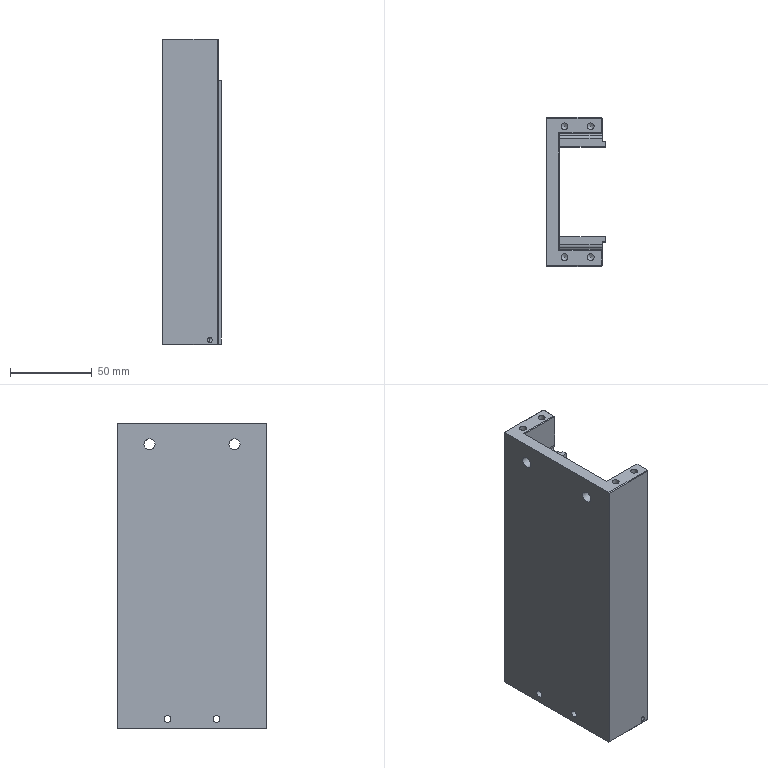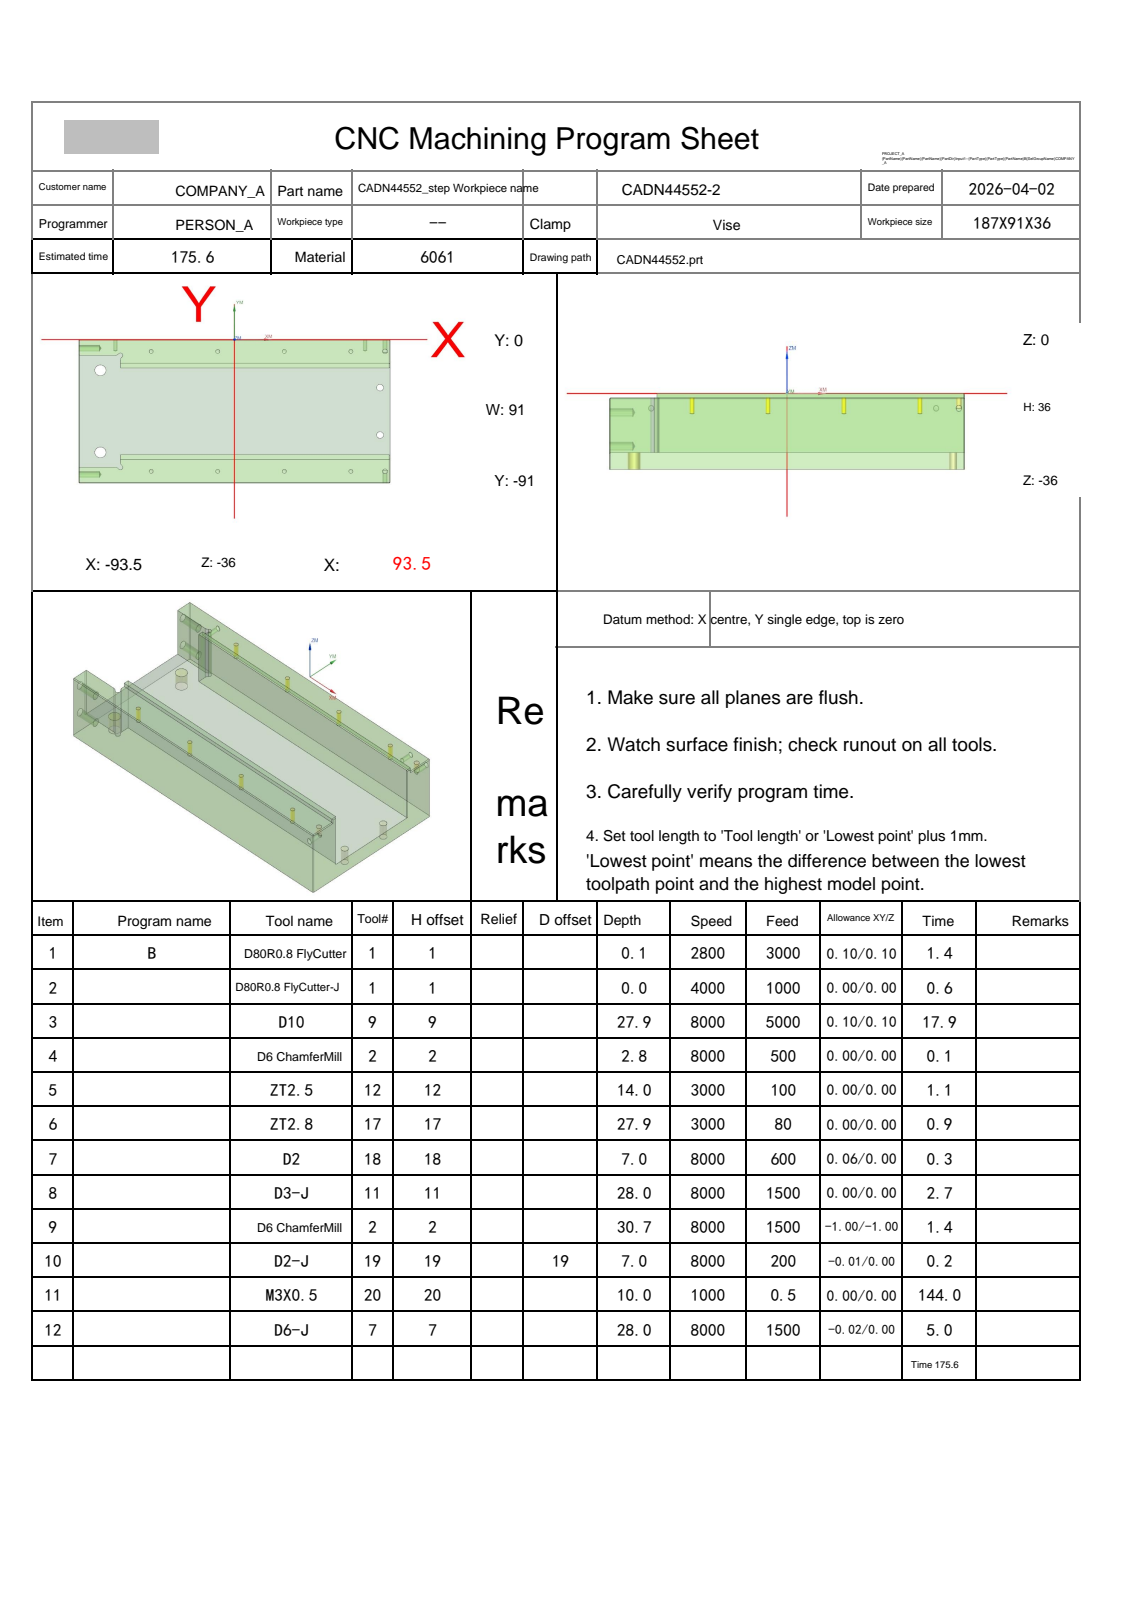NC program | NX | posted by the shop | part box 36 x 91 x 187 mm
Lines 5693 to 6699 of 12140:
N8 T11 M06
(D3-J  D=2.95 R=0. H=11 ce=0.00 di=0.00)
G00 G90 G54 X-74.719 Y-79.229 M03 S8000
G43 H11 Z20.
M08
Z-1.955
G01 X-74.718 Y-79.233 Z-2. F1500.
X-74.716 Y-79.243 Z-2.04
X-74.711 Y-79.26 Z-2.076
X-74.704 Y-79.281 Z-2.108
X-74.695 Y-79.306 Z-2.136
X-74.683 Y-79.333 Z-2.161
X-74.669 Y-79.362 Z-2.182
X-74.651 Y-79.392 Z-2.199
X-74.63 Y-79.421 Z-2.214
X-74.605 Y-79.448 Z-2.226
X-74.577 Y-79.473 Z-2.235
X-74.545 Y-79.494 Z-2.242
X-74.509 Y-79.511 Z-2.247
X-74.469 Y-79.521 Z-2.249
X-74.424 Y-79.525 Z-2.25
X-71.622
G02 X-68.52 Y-81.016 I0.0 J-3.975
G01 X-68.492 Y-81.034
X-68.466 Y-81.008
X-68.484 Y-80.98
G02 X-69.975 Y-77.877 I2.484 J3.103
G01 Y-75.076
X-69.989 Y-75.052 Z-2.251
X-70.03 Z-2.252
X-70.096 Y-75.076 Z-2.255
X-70.184 Y-75.12 Z-2.259
X-70.292 Y-75.183 Z-2.264
X-70.623 Y-75.411 Z-2.28
X-70.927 Y-75.64 Z-2.294
X-71.309 Y-75.946 Z-2.313
X-71.944 Y-76.503 Z-2.346
X-72.481 Y-77.019 Z-2.375
X-72.996 Y-77.555 Z-2.404
X-73.553 Y-78.19 Z-2.437
X-73.86 Y-78.572 Z-2.456
X-74.089 Y-78.876 Z-2.47
X-74.317 Y-79.208 Z-2.486
X-74.38 Y-79.316 Z-2.491
X-74.424 Y-79.404 Z-2.495
X-74.448 Y-79.47 Z-2.498
Y-79.511 Z-2.499
X-74.424 Y-79.525 Z-2.5
X-71.622
G02 X-68.52 Y-81.016 I0.0 J-3.975
G01 X-68.492 Y-81.034
X-68.466 Y-81.008
X-68.484 Y-80.98
G02 X-69.975 Y-77.877 I2.484 J3.103
G01 Y-75.076
X-69.989 Y-75.052 Z-2.501
X-70.03 Z-2.502
X-70.096 Y-75.076 Z-2.505
X-70.184 Y-75.12 Z-2.509
X-70.292 Y-75.183 Z-2.514
X-70.623 Y-75.411 Z-2.53
X-70.927 Y-75.64 Z-2.544
X-71.309 Y-75.946 Z-2.563
X-71.944 Y-76.503 Z-2.596
X-72.481 Y-77.019 Z-2.625
X-72.996 Y-77.555 Z-2.654
X-73.553 Y-78.19 Z-2.687
X-73.86 Y-78.572 Z-2.706
X-74.089 Y-78.876 Z-2.72
X-74.317 Y-79.208 Z-2.736
X-74.38 Y-79.316 Z-2.741
X-74.424 Y-79.404 Z-2.745
X-74.448 Y-79.47 Z-2.748
Y-79.511 Z-2.749
X-74.424 Y-79.525 Z-2.75
X-71.622
G02 X-68.52 Y-81.016 I0.0 J-3.975
G01 X-68.492 Y-81.034
X-68.466 Y-81.008
X-68.484 Y-80.98
G02 X-69.975 Y-77.877 I2.484 J3.103
G01 Y-75.076
X-69.989 Y-75.052 Z-2.751
X-70.03 Z-2.752
X-70.096 Y-75.076 Z-2.755
X-70.184 Y-75.12 Z-2.759
X-70.292 Y-75.183 Z-2.764
X-70.623 Y-75.411 Z-2.78
X-70.927 Y-75.64 Z-2.794
X-71.309 Y-75.946 Z-2.813
X-71.944 Y-76.503 Z-2.846
X-72.481 Y-77.019 Z-2.875
X-72.996 Y-77.555 Z-2.904
X-73.553 Y-78.19 Z-2.937
X-73.86 Y-78.572 Z-2.956
X-74.089 Y-78.876 Z-2.97
X-74.317 Y-79.208 Z-2.986
X-74.38 Y-79.316 Z-2.991
X-74.424 Y-79.404 Z-2.995
X-74.448 Y-79.47 Z-2.998
Y-79.511 Z-2.999
X-74.424 Y-79.525 Z-3.
X-71.622
G02 X-68.52 Y-81.016 I0.0 J-3.975
G01 X-68.492 Y-81.034
X-68.466 Y-81.008
X-68.484 Y-80.98
G02 X-69.975 Y-77.877 I2.484 J3.103
G01 Y-75.076
X-69.989 Y-75.052 Z-3.001
X-70.03 Z-3.002
X-70.096 Y-75.076 Z-3.005
X-70.184 Y-75.12 Z-3.009
X-70.292 Y-75.183 Z-3.014
X-70.623 Y-75.411 Z-3.03
X-70.927 Y-75.64 Z-3.044
X-71.309 Y-75.946 Z-3.063
X-71.944 Y-76.503 Z-3.096
X-72.481 Y-77.019 Z-3.125
X-72.996 Y-77.555 Z-3.154
X-73.553 Y-78.19 Z-3.187
X-73.86 Y-78.572 Z-3.206
X-74.089 Y-78.876 Z-3.22
X-74.317 Y-79.208 Z-3.236
X-74.38 Y-79.316 Z-3.241
X-74.424 Y-79.404 Z-3.245
X-74.448 Y-79.47 Z-3.248
Y-79.511 Z-3.249
X-74.424 Y-79.525 Z-3.25
X-71.622
G02 X-68.52 Y-81.016 I0.0 J-3.975
G01 X-68.492 Y-81.034
X-68.466 Y-81.008
X-68.484 Y-80.98
G02 X-69.975 Y-77.877 I2.484 J3.103
G01 Y-75.076
X-69.989 Y-75.052 Z-3.251
X-70.03 Z-3.252
X-70.096 Y-75.076 Z-3.255
X-70.184 Y-75.12 Z-3.259
X-70.292 Y-75.183 Z-3.264
X-70.623 Y-75.411 Z-3.28
X-70.927 Y-75.64 Z-3.294
X-71.309 Y-75.946 Z-3.313
X-71.944 Y-76.503 Z-3.346
X-72.481 Y-77.019 Z-3.375
X-72.996 Y-77.555 Z-3.404
X-73.553 Y-78.19 Z-3.437
X-73.86 Y-78.572 Z-3.456
X-74.089 Y-78.876 Z-3.47
X-74.317 Y-79.208 Z-3.486
X-74.38 Y-79.316 Z-3.491
X-74.424 Y-79.404 Z-3.495
X-74.448 Y-79.47 Z-3.498
Y-79.511 Z-3.499
X-74.424 Y-79.525 Z-3.5
X-71.622
G02 X-68.52 Y-81.016 I0.0 J-3.975
G01 X-68.492 Y-81.034
X-68.466 Y-81.008
X-68.484 Y-80.98
G02 X-69.975 Y-77.877 I2.484 J3.103
G01 Y-75.076
X-69.989 Y-75.052 Z-3.501
X-70.03 Z-3.502
X-70.096 Y-75.076 Z-3.505
X-70.184 Y-75.12 Z-3.509
X-70.292 Y-75.183 Z-3.514
X-70.623 Y-75.411 Z-3.53
X-70.927 Y-75.64 Z-3.544
X-71.309 Y-75.946 Z-3.563
X-71.944 Y-76.503 Z-3.596
X-72.481 Y-77.019 Z-3.625
X-72.996 Y-77.555 Z-3.654
X-73.553 Y-78.19 Z-3.687
X-73.86 Y-78.572 Z-3.706
X-74.089 Y-78.876 Z-3.72
X-74.317 Y-79.208 Z-3.736
X-74.38 Y-79.316 Z-3.741
X-74.424 Y-79.404 Z-3.745
X-74.448 Y-79.47 Z-3.748
Y-79.511 Z-3.749
X-74.424 Y-79.525 Z-3.75
X-71.622
G02 X-68.52 Y-81.016 I0.0 J-3.975
G01 X-68.492 Y-81.034
X-68.466 Y-81.008
X-68.484 Y-80.98
G02 X-69.975 Y-77.877 I2.484 J3.103
G01 Y-75.076
X-69.989 Y-75.052 Z-3.751
X-70.03 Z-3.752
X-70.096 Y-75.076 Z-3.755
X-70.184 Y-75.12 Z-3.759
X-70.292 Y-75.183 Z-3.764
X-70.623 Y-75.411 Z-3.78
X-70.927 Y-75.64 Z-3.794
X-71.309 Y-75.946 Z-3.813
X-71.944 Y-76.503 Z-3.846
X-72.481 Y-77.019 Z-3.875
X-72.996 Y-77.555 Z-3.904
X-73.553 Y-78.19 Z-3.937
X-73.86 Y-78.572 Z-3.956
X-74.089 Y-78.876 Z-3.97
X-74.317 Y-79.208 Z-3.986
X-74.38 Y-79.316 Z-3.991
X-74.424 Y-79.404 Z-3.995
X-74.448 Y-79.47 Z-3.998
Y-79.511 Z-3.999
X-74.424 Y-79.525 Z-4.
X-71.622
G02 X-68.52 Y-81.016 I0.0 J-3.975
G01 X-68.492 Y-81.034
X-68.466 Y-81.008
X-68.484 Y-80.98
G02 X-69.975 Y-77.877 I2.484 J3.103
G01 Y-75.076
X-69.989 Y-75.052 Z-4.001
X-70.03 Z-4.002
X-70.096 Y-75.076 Z-4.005
X-70.184 Y-75.12 Z-4.009
X-70.292 Y-75.183 Z-4.014
X-70.623 Y-75.411 Z-4.03
X-70.927 Y-75.64 Z-4.044
X-71.309 Y-75.946 Z-4.063
X-71.944 Y-76.503 Z-4.096
X-72.481 Y-77.019 Z-4.125
X-72.996 Y-77.555 Z-4.154
X-73.553 Y-78.19 Z-4.187
X-73.86 Y-78.572 Z-4.206
X-74.089 Y-78.876 Z-4.22
X-74.317 Y-79.208 Z-4.236
X-74.38 Y-79.316 Z-4.241
X-74.424 Y-79.404 Z-4.245
X-74.448 Y-79.47 Z-4.248
Y-79.511 Z-4.249
X-74.424 Y-79.525 Z-4.25
X-71.622
G02 X-68.52 Y-81.016 I0.0 J-3.975
G01 X-68.492 Y-81.034
X-68.466 Y-81.008
X-68.484 Y-80.98
G02 X-69.975 Y-77.877 I2.484 J3.103
G01 Y-75.076
X-69.989 Y-75.052 Z-4.251
X-70.03 Z-4.252
X-70.096 Y-75.076 Z-4.255
X-70.184 Y-75.12 Z-4.259
X-70.292 Y-75.183 Z-4.264
X-70.623 Y-75.411 Z-4.28
X-70.927 Y-75.64 Z-4.294
X-71.309 Y-75.946 Z-4.313
X-71.944 Y-76.503 Z-4.346
X-72.481 Y-77.019 Z-4.375
X-72.996 Y-77.555 Z-4.404
X-73.553 Y-78.19 Z-4.437
X-73.86 Y-78.572 Z-4.456
X-74.089 Y-78.876 Z-4.47
X-74.317 Y-79.208 Z-4.486
X-74.38 Y-79.316 Z-4.491
X-74.424 Y-79.404 Z-4.495
X-74.448 Y-79.47 Z-4.498
Y-79.511 Z-4.499
X-74.424 Y-79.525 Z-4.5
X-71.622
G02 X-68.52 Y-81.016 I0.0 J-3.975
G01 X-68.492 Y-81.034
X-68.466 Y-81.008
X-68.484 Y-80.98
G02 X-69.975 Y-77.877 I2.484 J3.103
G01 Y-75.076
X-69.989 Y-75.052 Z-4.501
X-70.03 Z-4.502
X-70.096 Y-75.076 Z-4.505
X-70.184 Y-75.12 Z-4.509
X-70.292 Y-75.183 Z-4.514
X-70.623 Y-75.411 Z-4.53
X-70.927 Y-75.64 Z-4.544
X-71.309 Y-75.946 Z-4.563
X-71.944 Y-76.503 Z-4.596
X-72.481 Y-77.019 Z-4.625
X-72.996 Y-77.555 Z-4.654
X-73.553 Y-78.19 Z-4.687
X-73.86 Y-78.572 Z-4.706
X-74.089 Y-78.876 Z-4.72
X-74.317 Y-79.208 Z-4.736
X-74.38 Y-79.316 Z-4.741
X-74.424 Y-79.404 Z-4.745
X-74.448 Y-79.47 Z-4.748
Y-79.511 Z-4.749
X-74.424 Y-79.525 Z-4.75
X-71.622
G02 X-68.52 Y-81.016 I0.0 J-3.975
G01 X-68.492 Y-81.034
X-68.466 Y-81.008
X-68.484 Y-80.98
G02 X-69.975 Y-77.877 I2.484 J3.103
G01 Y-75.076
X-69.989 Y-75.052 Z-4.751
X-70.03 Z-4.752
X-70.096 Y-75.076 Z-4.755
X-70.184 Y-75.12 Z-4.759
X-70.292 Y-75.183 Z-4.764
X-70.623 Y-75.411 Z-4.78
X-70.927 Y-75.64 Z-4.794
X-71.309 Y-75.946 Z-4.813
X-71.944 Y-76.503 Z-4.846
X-72.481 Y-77.019 Z-4.875
X-72.996 Y-77.555 Z-4.904
X-73.553 Y-78.19 Z-4.937
X-73.86 Y-78.572 Z-4.956
X-74.089 Y-78.876 Z-4.97
X-74.317 Y-79.208 Z-4.986
X-74.38 Y-79.316 Z-4.991
X-74.424 Y-79.404 Z-4.995
X-74.448 Y-79.47 Z-4.998
Y-79.511 Z-4.999
X-74.424 Y-79.525 Z-5.
X-71.622
G02 X-68.52 Y-81.016 I0.0 J-3.975
G01 X-68.492 Y-81.034
X-68.466 Y-81.008
X-68.484 Y-80.98
G02 X-69.975 Y-77.877 I2.484 J3.103
G01 Y-75.076
X-69.989 Y-75.052 Z-5.001
X-70.03 Z-5.002
X-70.096 Y-75.076 Z-5.005
X-70.184 Y-75.12 Z-5.009
X-70.292 Y-75.183 Z-5.014
X-70.623 Y-75.411 Z-5.03
X-70.927 Y-75.64 Z-5.044
X-71.309 Y-75.946 Z-5.063
X-71.944 Y-76.503 Z-5.096
X-72.481 Y-77.019 Z-5.125
X-72.996 Y-77.555 Z-5.154
X-73.553 Y-78.19 Z-5.187
X-73.86 Y-78.572 Z-5.206
X-74.089 Y-78.876 Z-5.22
X-74.317 Y-79.208 Z-5.236
X-74.38 Y-79.316 Z-5.241
X-74.424 Y-79.404 Z-5.245
X-74.448 Y-79.47 Z-5.248
Y-79.511 Z-5.249
X-74.424 Y-79.525 Z-5.25
X-71.622
G02 X-68.52 Y-81.016 I0.0 J-3.975
G01 X-68.492 Y-81.034
X-68.466 Y-81.008
X-68.484 Y-80.98
G02 X-69.975 Y-77.877 I2.484 J3.103
G01 Y-75.076
X-69.989 Y-75.052 Z-5.251
X-70.03 Z-5.252
X-70.096 Y-75.076 Z-5.255
X-70.184 Y-75.12 Z-5.259
X-70.292 Y-75.183 Z-5.264
X-70.623 Y-75.411 Z-5.28
X-70.927 Y-75.64 Z-5.294
X-71.309 Y-75.946 Z-5.313
X-71.944 Y-76.503 Z-5.346
X-72.481 Y-77.019 Z-5.375
X-72.996 Y-77.555 Z-5.404
X-73.553 Y-78.19 Z-5.437
X-73.86 Y-78.572 Z-5.456
X-74.089 Y-78.876 Z-5.47
X-74.317 Y-79.208 Z-5.486
X-74.38 Y-79.316 Z-5.491
X-74.424 Y-79.404 Z-5.495
X-74.448 Y-79.47 Z-5.498
Y-79.511 Z-5.499
X-74.424 Y-79.525 Z-5.5
X-71.622
G02 X-68.52 Y-81.016 I0.0 J-3.975
G01 X-68.492 Y-81.034
X-68.466 Y-81.008
X-68.484 Y-80.98
G02 X-69.975 Y-77.877 I2.484 J3.103
G01 Y-75.076
X-69.989 Y-75.052 Z-5.501
X-70.03 Z-5.502
X-70.096 Y-75.076 Z-5.505
X-70.184 Y-75.12 Z-5.509
X-70.292 Y-75.183 Z-5.514
X-70.623 Y-75.411 Z-5.53
X-70.927 Y-75.64 Z-5.544
X-71.309 Y-75.946 Z-5.563
X-71.944 Y-76.503 Z-5.596
X-72.481 Y-77.019 Z-5.625
X-72.996 Y-77.555 Z-5.654
X-73.553 Y-78.19 Z-5.687
X-73.86 Y-78.572 Z-5.706
X-74.089 Y-78.876 Z-5.72
X-74.317 Y-79.208 Z-5.736
X-74.38 Y-79.316 Z-5.741
X-74.424 Y-79.404 Z-5.745
X-74.448 Y-79.47 Z-5.748
Y-79.511 Z-5.749
X-74.424 Y-79.525 Z-5.75
X-71.622
G02 X-68.52 Y-81.016 I0.0 J-3.975
G01 X-68.492 Y-81.034
X-68.466 Y-81.008
X-68.484 Y-80.98
G02 X-69.975 Y-77.877 I2.484 J3.103
G01 Y-75.076
X-69.989 Y-75.052 Z-5.751
X-70.03 Z-5.752
X-70.096 Y-75.076 Z-5.755
X-70.184 Y-75.12 Z-5.759
X-70.292 Y-75.183 Z-5.764
X-70.623 Y-75.411 Z-5.78
X-70.927 Y-75.64 Z-5.794
X-71.309 Y-75.946 Z-5.813
X-71.944 Y-76.503 Z-5.846
X-72.481 Y-77.019 Z-5.875
X-72.996 Y-77.555 Z-5.904
X-73.553 Y-78.19 Z-5.937
X-73.86 Y-78.572 Z-5.956
X-74.089 Y-78.876 Z-5.97
X-74.317 Y-79.208 Z-5.986
X-74.38 Y-79.316 Z-5.991
X-74.424 Y-79.404 Z-5.995
X-74.448 Y-79.47 Z-5.998
Y-79.511 Z-5.999
X-74.424 Y-79.525 Z-6.
X-71.622
G02 X-68.52 Y-81.016 I0.0 J-3.975
G01 X-68.492 Y-81.034
X-68.466 Y-81.008
X-68.484 Y-80.98
G02 X-69.975 Y-77.877 I2.484 J3.103
G01 Y-75.076
X-69.989 Y-75.052 Z-6.001
X-70.03 Z-6.002
X-70.096 Y-75.076 Z-6.005
X-70.184 Y-75.12 Z-6.009
X-70.292 Y-75.183 Z-6.014
X-70.623 Y-75.411 Z-6.03
X-70.927 Y-75.64 Z-6.044
X-71.309 Y-75.946 Z-6.063
X-71.944 Y-76.503 Z-6.096
X-72.481 Y-77.019 Z-6.125
X-72.996 Y-77.555 Z-6.154
X-73.553 Y-78.19 Z-6.187
X-73.86 Y-78.572 Z-6.206
X-74.089 Y-78.876 Z-6.22
X-74.317 Y-79.208 Z-6.236
X-74.38 Y-79.316 Z-6.241
X-74.424 Y-79.404 Z-6.245
X-74.448 Y-79.47 Z-6.248
Y-79.511 Z-6.249
X-74.424 Y-79.525 Z-6.25
X-71.622
G02 X-68.52 Y-81.016 I0.0 J-3.975
G01 X-68.492 Y-81.034
X-68.466 Y-81.008
X-68.484 Y-80.98
G02 X-69.975 Y-77.877 I2.484 J3.103
G01 Y-75.076
X-69.989 Y-75.052 Z-6.251
X-70.03 Z-6.252
X-70.096 Y-75.076 Z-6.255
X-70.184 Y-75.12 Z-6.259
X-70.292 Y-75.183 Z-6.264
X-70.623 Y-75.411 Z-6.28
X-70.927 Y-75.64 Z-6.294
X-71.309 Y-75.946 Z-6.313
X-71.944 Y-76.503 Z-6.346
X-72.481 Y-77.019 Z-6.375
X-72.996 Y-77.555 Z-6.404
X-73.553 Y-78.19 Z-6.437
X-73.86 Y-78.572 Z-6.456
X-74.089 Y-78.876 Z-6.47
X-74.317 Y-79.208 Z-6.486
X-74.38 Y-79.316 Z-6.491
X-74.424 Y-79.404 Z-6.495
X-74.448 Y-79.47 Z-6.498
Y-79.511 Z-6.499
X-74.424 Y-79.525 Z-6.5
X-71.622
G02 X-68.52 Y-81.016 I0.0 J-3.975
G01 X-68.492 Y-81.034
X-68.466 Y-81.008
X-68.484 Y-80.98
G02 X-69.975 Y-77.877 I2.484 J3.103
G01 Y-75.076
X-69.989 Y-75.052 Z-6.501
X-70.03 Z-6.502
X-70.096 Y-75.076 Z-6.505
X-70.184 Y-75.12 Z-6.509
X-70.292 Y-75.183 Z-6.514
X-70.623 Y-75.411 Z-6.53
X-70.927 Y-75.64 Z-6.544
X-71.309 Y-75.946 Z-6.563
X-71.944 Y-76.503 Z-6.596
X-72.481 Y-77.019 Z-6.625
X-72.996 Y-77.555 Z-6.654
X-73.553 Y-78.19 Z-6.687
X-73.86 Y-78.572 Z-6.706
X-74.089 Y-78.876 Z-6.72
X-74.317 Y-79.208 Z-6.736
X-74.38 Y-79.316 Z-6.741
X-74.424 Y-79.404 Z-6.745
X-74.448 Y-79.47 Z-6.748
Y-79.511 Z-6.749
X-74.424 Y-79.525 Z-6.75
X-71.622
G02 X-68.52 Y-81.016 I0.0 J-3.975
G01 X-68.492 Y-81.034
X-68.466 Y-81.008
X-68.484 Y-80.98
G02 X-69.975 Y-77.877 I2.484 J3.103
G01 Y-75.076
X-69.989 Y-75.052 Z-6.751
X-70.03 Z-6.752
X-70.096 Y-75.076 Z-6.755
X-70.184 Y-75.12 Z-6.759
X-70.292 Y-75.183 Z-6.764
X-70.623 Y-75.411 Z-6.78
X-70.927 Y-75.64 Z-6.794
X-71.309 Y-75.946 Z-6.813
X-71.944 Y-76.503 Z-6.846
X-72.481 Y-77.019 Z-6.875
X-72.996 Y-77.555 Z-6.904
X-73.553 Y-78.19 Z-6.937
X-73.86 Y-78.572 Z-6.956
X-74.089 Y-78.876 Z-6.97
X-74.317 Y-79.208 Z-6.986
X-74.38 Y-79.316 Z-6.991
X-74.424 Y-79.404 Z-6.995
X-74.448 Y-79.47 Z-6.998
Y-79.511 Z-6.999
X-74.424 Y-79.525 Z-7.
X-71.622
G02 X-68.52 Y-81.016 I0.0 J-3.975
G01 X-68.492 Y-81.034
X-68.466 Y-81.008
X-68.484 Y-80.98
G02 X-69.975 Y-77.877 I2.484 J3.103
G01 Y-75.076
X-69.989 Y-75.052 Z-7.001
X-70.03 Z-7.002
X-70.096 Y-75.076 Z-7.005
X-70.184 Y-75.12 Z-7.009
X-70.292 Y-75.183 Z-7.014
X-70.623 Y-75.411 Z-7.03
X-70.927 Y-75.64 Z-7.044
X-71.309 Y-75.946 Z-7.063
X-71.944 Y-76.503 Z-7.096
X-72.481 Y-77.019 Z-7.125
X-72.996 Y-77.555 Z-7.154
X-73.553 Y-78.19 Z-7.187
X-73.86 Y-78.572 Z-7.206
X-74.089 Y-78.876 Z-7.22
X-74.317 Y-79.208 Z-7.236
X-74.38 Y-79.316 Z-7.241
X-74.424 Y-79.404 Z-7.245
X-74.448 Y-79.47 Z-7.248
Y-79.511 Z-7.249
X-74.424 Y-79.525 Z-7.25
X-71.622
G02 X-68.52 Y-81.016 I0.0 J-3.975
G01 X-68.492 Y-81.034
X-68.466 Y-81.008
X-68.484 Y-80.98
G02 X-69.975 Y-77.877 I2.484 J3.103
G01 Y-75.076
X-69.989 Y-75.052 Z-7.251
X-70.03 Z-7.252
X-70.096 Y-75.076 Z-7.255
X-70.184 Y-75.12 Z-7.259
X-70.292 Y-75.183 Z-7.264
X-70.623 Y-75.411 Z-7.28
X-70.927 Y-75.64 Z-7.294
X-71.309 Y-75.946 Z-7.313
X-71.944 Y-76.503 Z-7.346
X-72.481 Y-77.019 Z-7.375
X-72.996 Y-77.555 Z-7.404
X-73.553 Y-78.19 Z-7.437
X-73.86 Y-78.572 Z-7.456
X-74.089 Y-78.876 Z-7.47
X-74.317 Y-79.208 Z-7.486
X-74.38 Y-79.316 Z-7.491
X-74.424 Y-79.404 Z-7.495
X-74.448 Y-79.47 Z-7.498
Y-79.511 Z-7.499
X-74.424 Y-79.525 Z-7.5
X-71.622
G02 X-68.52 Y-81.016 I0.0 J-3.975
G01 X-68.492 Y-81.034
X-68.466 Y-81.008
X-68.484 Y-80.98
G02 X-69.975 Y-77.877 I2.484 J3.103
G01 Y-75.076
X-69.989 Y-75.052 Z-7.501
X-70.03 Z-7.502
X-70.096 Y-75.076 Z-7.505
X-70.184 Y-75.12 Z-7.509
X-70.292 Y-75.183 Z-7.514
X-70.623 Y-75.411 Z-7.53
X-70.927 Y-75.64 Z-7.544
X-71.309 Y-75.946 Z-7.563
X-71.944 Y-76.503 Z-7.596
X-72.481 Y-77.019 Z-7.625
X-72.996 Y-77.555 Z-7.654
X-73.553 Y-78.19 Z-7.687
X-73.86 Y-78.572 Z-7.706
X-74.089 Y-78.876 Z-7.72
X-74.317 Y-79.208 Z-7.736
X-74.38 Y-79.316 Z-7.741
X-74.424 Y-79.404 Z-7.745
X-74.448 Y-79.47 Z-7.748
Y-79.511 Z-7.749
X-74.424 Y-79.525 Z-7.75
X-71.622
G02 X-68.52 Y-81.016 I0.0 J-3.975
G01 X-68.492 Y-81.034
X-68.466 Y-81.008
X-68.484 Y-80.98
G02 X-69.975 Y-77.877 I2.484 J3.103
G01 Y-75.076
X-69.989 Y-75.052 Z-7.751
X-70.03 Z-7.752
X-70.096 Y-75.076 Z-7.755
X-70.184 Y-75.12 Z-7.759
X-70.292 Y-75.183 Z-7.764
X-70.623 Y-75.411 Z-7.78
X-70.927 Y-75.64 Z-7.794
X-71.309 Y-75.946 Z-7.813
X-71.944 Y-76.503 Z-7.846
X-72.481 Y-77.019 Z-7.875
X-72.996 Y-77.555 Z-7.904
X-73.553 Y-78.19 Z-7.937
X-73.86 Y-78.572 Z-7.956
X-74.089 Y-78.876 Z-7.97
X-74.317 Y-79.208 Z-7.986
X-74.38 Y-79.316 Z-7.991
X-74.424 Y-79.404 Z-7.995
X-74.448 Y-79.47 Z-7.998
Y-79.511 Z-7.999
X-74.424 Y-79.525 Z-8.
X-71.622
G02 X-68.52 Y-81.016 I0.0 J-3.975
G01 X-68.492 Y-81.034
X-68.466 Y-81.008
X-68.484 Y-80.98
G02 X-69.975 Y-77.877 I2.484 J3.103
G01 Y-75.076
X-69.989 Y-75.052 Z-8.001
X-70.03 Z-8.002
X-70.096 Y-75.076 Z-8.005
X-70.184 Y-75.12 Z-8.009
X-70.292 Y-75.183 Z-8.014
X-70.623 Y-75.411 Z-8.03
X-70.927 Y-75.64 Z-8.044
X-71.309 Y-75.946 Z-8.063
X-71.944 Y-76.503 Z-8.096
X-72.481 Y-77.019 Z-8.125
X-72.996 Y-77.555 Z-8.154
X-73.553 Y-78.19 Z-8.187
X-73.86 Y-78.572 Z-8.206
X-74.089 Y-78.876 Z-8.22
X-74.317 Y-79.208 Z-8.236
X-74.38 Y-79.316 Z-8.241
X-74.424 Y-79.404 Z-8.245
X-74.448 Y-79.47 Z-8.248
Y-79.511 Z-8.249
X-74.424 Y-79.525 Z-8.25
X-71.622
G02 X-68.52 Y-81.016 I0.0 J-3.975
G01 X-68.492 Y-81.034
X-68.466 Y-81.008
X-68.484 Y-80.98
G02 X-69.975 Y-77.877 I2.484 J3.103
G01 Y-75.076
X-69.989 Y-75.052 Z-8.251
X-70.03 Z-8.252
X-70.096 Y-75.076 Z-8.255
X-70.184 Y-75.12 Z-8.259
X-70.292 Y-75.183 Z-8.264
X-70.623 Y-75.411 Z-8.28
X-70.927 Y-75.64 Z-8.294
X-71.309 Y-75.946 Z-8.313
X-71.944 Y-76.503 Z-8.346
X-72.481 Y-77.019 Z-8.375
X-72.996 Y-77.555 Z-8.404
X-73.553 Y-78.19 Z-8.437
X-73.86 Y-78.572 Z-8.456
X-74.089 Y-78.876 Z-8.47
X-74.317 Y-79.208 Z-8.486
X-74.38 Y-79.316 Z-8.491
X-74.424 Y-79.404 Z-8.495
X-74.448 Y-79.47 Z-8.498
Y-79.511 Z-8.499
X-74.424 Y-79.525 Z-8.5
X-71.622
G02 X-68.52 Y-81.016 I0.0 J-3.975
G01 X-68.492 Y-81.034
X-68.466 Y-81.008
X-68.484 Y-80.98
G02 X-69.975 Y-77.877 I2.484 J3.103
G01 Y-75.076
X-69.989 Y-75.052 Z-8.501
X-70.03 Z-8.502
X-70.096 Y-75.076 Z-8.505
X-70.184 Y-75.12 Z-8.509
X-70.292 Y-75.183 Z-8.514
X-70.623 Y-75.411 Z-8.53
X-70.927 Y-75.64 Z-8.544
X-71.309 Y-75.946 Z-8.563
X-71.944 Y-76.503 Z-8.596
X-72.481 Y-77.019 Z-8.625
X-72.996 Y-77.555 Z-8.654
X-73.553 Y-78.19 Z-8.687
X-73.86 Y-78.572 Z-8.706
X-74.089 Y-78.876 Z-8.72
X-74.317 Y-79.208 Z-8.736
X-74.38 Y-79.316 Z-8.741
X-74.424 Y-79.404 Z-8.745
X-74.448 Y-79.47 Z-8.748
Y-79.511 Z-8.749
X-74.424 Y-79.525 Z-8.75
X-71.622
G02 X-68.52 Y-81.016 I0.0 J-3.975
G01 X-68.492 Y-81.034
X-68.466 Y-81.008
X-68.484 Y-80.98
G02 X-69.975 Y-77.877 I2.484 J3.103
G01 Y-75.076
X-69.989 Y-75.052 Z-8.751
X-70.03 Z-8.752
X-70.096 Y-75.076 Z-8.755
X-70.184 Y-75.12 Z-8.759
X-70.292 Y-75.183 Z-8.764
X-70.623 Y-75.411 Z-8.78
X-70.927 Y-75.64 Z-8.794
X-71.309 Y-75.946 Z-8.813
X-71.944 Y-76.503 Z-8.846
X-72.481 Y-77.019 Z-8.875
X-72.996 Y-77.555 Z-8.904
X-73.553 Y-78.19 Z-8.937
X-73.86 Y-78.572 Z-8.956
X-74.089 Y-78.876 Z-8.97
X-74.317 Y-79.208 Z-8.986
X-74.38 Y-79.316 Z-8.991
X-74.424 Y-79.404 Z-8.995
X-74.448 Y-79.47 Z-8.998
Y-79.511 Z-8.999
X-74.424 Y-79.525 Z-9.
X-71.622
G02 X-68.52 Y-81.016 I0.0 J-3.975
G01 X-68.492 Y-81.034
X-68.466 Y-81.008
X-68.484 Y-80.98
G02 X-69.975 Y-77.877 I2.484 J3.103
G01 Y-75.076
X-69.989 Y-75.052 Z-9.001
X-70.03 Z-9.002
X-70.096 Y-75.076 Z-9.005
X-70.184 Y-75.12 Z-9.009
X-70.292 Y-75.183 Z-9.014
X-70.623 Y-75.411 Z-9.03
X-70.927 Y-75.64 Z-9.044
X-71.309 Y-75.946 Z-9.063
X-71.944 Y-76.503 Z-9.096
X-72.481 Y-77.019 Z-9.125
X-72.996 Y-77.555 Z-9.154
X-73.553 Y-78.19 Z-9.187
X-73.86 Y-78.572 Z-9.206
X-74.089 Y-78.876 Z-9.22
X-74.317 Y-79.208 Z-9.236
X-74.38 Y-79.316 Z-9.241
X-74.424 Y-79.404 Z-9.245
X-74.448 Y-79.47 Z-9.248
Y-79.511 Z-9.249
X-74.424 Y-79.525 Z-9.25
X-71.622
G02 X-68.52 Y-81.016 I0.0 J-3.975
G01 X-68.492 Y-81.034
X-68.466 Y-81.008
X-68.484 Y-80.98
G02 X-69.975 Y-77.877 I2.484 J3.103
G01 Y-75.076
X-69.989 Y-75.052 Z-9.251
X-70.03 Z-9.252
X-70.096 Y-75.076 Z-9.255
X-70.184 Y-75.12 Z-9.259
X-70.292 Y-75.183 Z-9.264
X-70.623 Y-75.411 Z-9.28
X-70.927 Y-75.64 Z-9.294
X-71.309 Y-75.946 Z-9.313
X-71.944 Y-76.503 Z-9.346
X-72.481 Y-77.019 Z-9.375
X-72.996 Y-77.555 Z-9.404
X-73.553 Y-78.19 Z-9.437
X-73.86 Y-78.572 Z-9.456
X-74.089 Y-78.876 Z-9.47
X-74.317 Y-79.208 Z-9.486
X-74.38 Y-79.316 Z-9.491
X-74.424 Y-79.404 Z-9.495
X-74.448 Y-79.47 Z-9.498
Y-79.511 Z-9.499
X-74.424 Y-79.525 Z-9.5
X-71.622
G02 X-68.52 Y-81.016 I0.0 J-3.975
G01 X-68.492 Y-81.034
X-68.466 Y-81.008
X-68.484 Y-80.98
G02 X-69.975 Y-77.877 I2.484 J3.103
G01 Y-75.076
X-69.989 Y-75.052 Z-9.501
X-70.03 Z-9.502
X-70.096 Y-75.076 Z-9.505
X-70.184 Y-75.12 Z-9.509
X-70.292 Y-75.183 Z-9.514
X-70.623 Y-75.411 Z-9.53
X-70.927 Y-75.64 Z-9.544
X-71.309 Y-75.946 Z-9.563
X-71.944 Y-76.503 Z-9.596
X-72.481 Y-77.019 Z-9.625
X-72.996 Y-77.555 Z-9.654
X-73.553 Y-78.19 Z-9.687
X-73.86 Y-78.572 Z-9.706
X-74.089 Y-78.876 Z-9.72
X-74.317 Y-79.208 Z-9.736
X-74.38 Y-79.316 Z-9.741
X-74.424 Y-79.404 Z-9.745
X-74.448 Y-79.47 Z-9.748
Y-79.511 Z-9.749
X-74.424 Y-79.525 Z-9.75
X-71.622
G02 X-68.52 Y-81.016 I0.0 J-3.975
G01 X-68.492 Y-81.034
X-68.466 Y-81.008
X-68.484 Y-80.98
G02 X-69.975 Y-77.877 I2.484 J3.103
G01 Y-75.076
X-69.989 Y-75.052 Z-9.751
X-70.03 Z-9.752
X-70.096 Y-75.076 Z-9.755
X-70.184 Y-75.12 Z-9.759
X-70.292 Y-75.183 Z-9.764
X-70.623 Y-75.411 Z-9.78
X-70.927 Y-75.64 Z-9.794
X-71.309 Y-75.946 Z-9.813
X-71.944 Y-76.503 Z-9.846
X-72.481 Y-77.019 Z-9.875
X-72.996 Y-77.555 Z-9.904
X-73.553 Y-78.19 Z-9.937
X-73.86 Y-78.572 Z-9.956
X-74.089 Y-78.876 Z-9.97
X-74.317 Y-79.208 Z-9.986
X-74.38 Y-79.316 Z-9.991
X-74.424 Y-79.404 Z-9.995
X-74.448 Y-79.47 Z-9.998
Y-79.511 Z-9.999
X-74.424 Y-79.525 Z-10.
X-71.622
G02 X-68.52 Y-81.016 I0.0 J-3.975
G01 X-68.492 Y-81.034
X-68.466 Y-81.008
X-68.484 Y-80.98
G02 X-69.975 Y-77.877 I2.484 J3.103
G01 Y-75.076
X-69.989 Y-75.052 Z-10.001
X-70.03 Z-10.002
X-70.096 Y-75.076 Z-10.005
X-70.184 Y-75.12 Z-10.009
X-70.292 Y-75.183 Z-10.014
X-70.623 Y-75.411 Z-10.03
X-70.927 Y-75.64 Z-10.044
X-71.309 Y-75.946 Z-10.063
X-71.944 Y-76.503 Z-10.096
X-72.481 Y-77.019 Z-10.125
X-72.996 Y-77.555 Z-10.154
X-73.553 Y-78.19 Z-10.187
X-73.86 Y-78.572 Z-10.206
X-74.089 Y-78.876 Z-10.22
X-74.317 Y-79.208 Z-10.236
X-74.38 Y-79.316 Z-10.241
X-74.424 Y-79.404 Z-10.245
X-74.448 Y-79.47 Z-10.248
Y-79.511 Z-10.249
X-74.424 Y-79.525 Z-10.25
X-71.622
G02 X-68.52 Y-81.016 I0.0 J-3.975
G01 X-68.492 Y-81.034
X-68.466 Y-81.008
X-68.484 Y-80.98
G02 X-69.975 Y-77.877 I2.484 J3.103
G01 Y-75.076
X-69.989 Y-75.052 Z-10.251
X-70.03 Z-10.252
X-70.096 Y-75.076 Z-10.255
X-70.184 Y-75.12 Z-10.259
X-70.292 Y-75.183 Z-10.264
X-70.623 Y-75.411 Z-10.28
X-70.927 Y-75.64 Z-10.294
X-71.309 Y-75.946 Z-10.313
X-71.944 Y-76.503 Z-10.346
X-72.481 Y-77.019 Z-10.375
X-72.996 Y-77.555 Z-10.404
X-73.553 Y-78.19 Z-10.437
X-73.86 Y-78.572 Z-10.456
X-74.089 Y-78.876 Z-10.47
X-74.317 Y-79.208 Z-10.486
X-74.38 Y-79.316 Z-10.491
X-74.424 Y-79.404 Z-10.495
X-74.448 Y-79.47 Z-10.498
Y-79.511 Z-10.499
X-74.424 Y-79.525 Z-10.5
X-71.622
G02 X-68.52 Y-81.016 I0.0 J-3.975
G01 X-68.492 Y-81.034
X-68.466 Y-81.008
X-68.484 Y-80.98
G02 X-69.975 Y-77.877 I2.484 J3.103
G01 Y-75.076
X-69.989 Y-75.052 Z-10.501
X-70.03 Z-10.502
X-70.096 Y-75.076 Z-10.505
X-70.184 Y-75.12 Z-10.509
X-70.292 Y-75.183 Z-10.514
X-70.623 Y-75.411 Z-10.53
X-70.927 Y-75.64 Z-10.544
X-71.309 Y-75.946 Z-10.563
X-71.944 Y-76.503 Z-10.596
X-72.481 Y-77.019 Z-10.625
X-72.996 Y-77.555 Z-10.654
X-73.553 Y-78.19 Z-10.687
X-73.86 Y-78.572 Z-10.706
X-74.089 Y-78.876 Z-10.72
X-74.317 Y-79.208 Z-10.736
X-74.38 Y-79.316 Z-10.741
X-74.424 Y-79.404 Z-10.745
X-74.448 Y-79.47 Z-10.748
Y-79.511 Z-10.749
X-74.424 Y-79.525 Z-10.75
X-71.622
G02 X-68.52 Y-81.016 I0.0 J-3.975
G01 X-68.492 Y-81.034
X-68.466 Y-81.008
X-68.484 Y-80.98
G02 X-69.975 Y-77.877 I2.484 J3.103
G01 Y-75.076
X-69.989 Y-75.052 Z-10.751
X-70.03 Z-10.752
X-70.096 Y-75.076 Z-10.755
X-70.184 Y-75.12 Z-10.759
X-70.292 Y-75.183 Z-10.764
X-70.623 Y-75.411 Z-10.78
X-70.927 Y-75.64 Z-10.794
X-71.309 Y-75.946 Z-10.813
X-71.944 Y-76.503 Z-10.846
X-72.481 Y-77.019 Z-10.875
X-72.996 Y-77.555 Z-10.904
X-73.553 Y-78.19 Z-10.937
X-73.86 Y-78.572 Z-10.956
X-74.089 Y-78.876 Z-10.97
X-74.317 Y-79.208 Z-10.986
X-74.38 Y-79.316 Z-10.991
X-74.424 Y-79.404 Z-10.995
X-74.448 Y-79.47 Z-10.998
Y-79.511 Z-10.999
X-74.424 Y-79.525 Z-11.
X-71.622
G02 X-68.52 Y-81.016 I0.0 J-3.975
G01 X-68.492 Y-81.034
X-68.466 Y-81.008
X-68.484 Y-80.98
G02 X-69.975 Y-77.877 I2.484 J3.103
G01 Y-75.076
X-69.989 Y-75.052 Z-11.001
X-70.03 Z-11.002
X-70.096 Y-75.076 Z-11.005
X-70.184 Y-75.12 Z-11.009
X-70.292 Y-75.183 Z-11.014
X-70.623 Y-75.411 Z-11.03
X-70.927 Y-75.64 Z-11.044
X-71.309 Y-75.946 Z-11.063
X-71.944 Y-76.503 Z-11.096
X-72.481 Y-77.019 Z-11.125
X-72.996 Y-77.555 Z-11.154
X-73.553 Y-78.19 Z-11.187
X-73.86 Y-78.572 Z-11.206
X-74.089 Y-78.876 Z-11.22
X-74.317 Y-79.208 Z-11.236
X-74.38 Y-79.316 Z-11.241
X-74.424 Y-79.404 Z-11.245
X-74.448 Y-79.47 Z-11.248
Y-79.511 Z-11.249
X-74.424 Y-79.525 Z-11.25
X-71.622
G02 X-68.52 Y-81.016 I0.0 J-3.975
G01 X-68.492 Y-81.034
X-68.466 Y-81.008
X-68.484 Y-80.98
G02 X-69.975 Y-77.877 I2.484 J3.103
G01 Y-75.076
X-69.989 Y-75.052 Z-11.251
X-70.03 Z-11.252
X-70.096 Y-75.076 Z-11.255
X-70.184 Y-75.12 Z-11.259
X-70.292 Y-75.183 Z-11.264
X-70.623 Y-75.411 Z-11.28
X-70.927 Y-75.64 Z-11.294